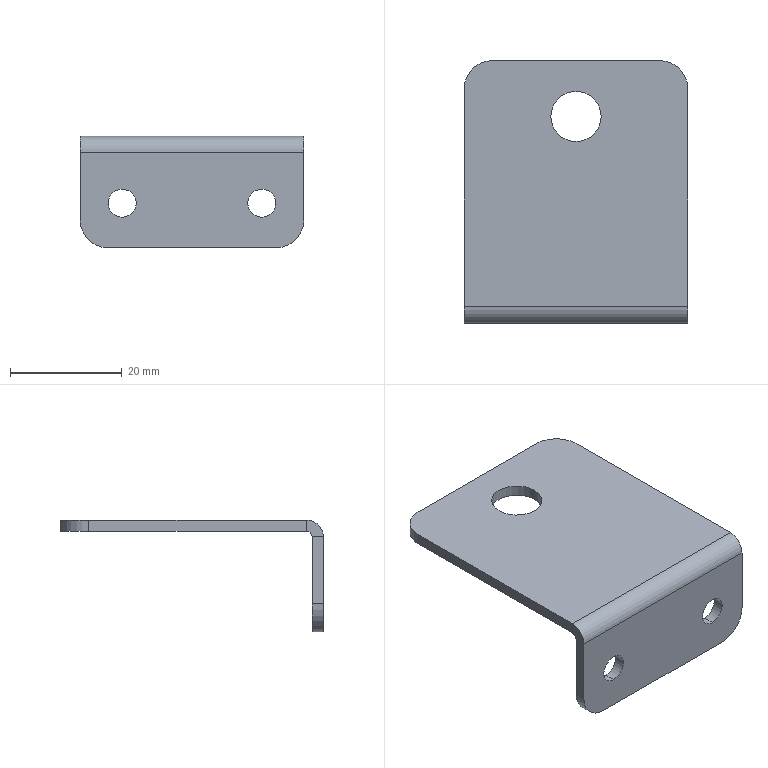Part | SolidWorks | features BaseBody 1 | 1 solid | 24 faces | box 40 x 47 x 20 mm | volume 4883 mm3 | cylinder 12 | plane 12 | commonest cylinder face diameters 5 x4 10 x4 9 x2 2 x1 6 x1
STEP:
#1=CARTESIAN_POINT('',(-12.5,-21.5,-9.5));
#2=VERTEX_POINT('',#1);
#3=CARTESIAN_POINT('',(-12.5,-23.5,-9.5));
#4=VERTEX_POINT('',#3);
#5=CARTESIAN_POINT('',(-12.5,-21.5,-9.5));
#6=DIRECTION('',(0.,-1.,0.));
#7=VECTOR('',#6,1000.);
#8=LINE('',#5,#7);
#9=EDGE_CURVE('',#2,#4,#8,.T.);
#10=ORIENTED_EDGE('',*,*,#9,.F.);
#11=CARTESIAN_POINT('',(-12.5,-21.5,-14.5));
#12=VERTEX_POINT('',#11);
#13=CARTESIAN_POINT('',(-12.5,-21.5,-12.));
#14=DIRECTION('',(0.,-1.,0.));
#15=DIRECTION('',(0.,0.,-1.));
#16=AXIS2_PLACEMENT_3D('',#13,#14,#15);
#17=CIRCLE('',#16,2.5);
#18=EDGE_CURVE('',#12,#2,#17,.T.);
#19=ORIENTED_EDGE('',*,*,#18,.F.);
#20=CARTESIAN_POINT('',(-12.5,-23.5,-14.5));
#21=VERTEX_POINT('',#20);
#22=CARTESIAN_POINT('',(-12.5,-21.5,-14.5));
#23=DIRECTION('',(0.,-1.,0.));
#24=VECTOR('',#23,1000.);
#25=LINE('',#22,#24);
#26=EDGE_CURVE('',#12,#21,#25,.T.);
#27=ORIENTED_EDGE('',*,*,#26,.T.);
#28=CARTESIAN_POINT('',(-12.5,-23.5,-12.));
#29=DIRECTION('',(0.,-1.,0.));
#30=DIRECTION('',(0.,0.,-1.));
#31=AXIS2_PLACEMENT_3D('',#28,#29,#30);
#32=CIRCLE('',#31,2.5);
#33=EDGE_CURVE('',#21,#4,#32,.T.);
#34=ORIENTED_EDGE('',*,*,#33,.T.);
#35=EDGE_LOOP('',(#10,#19,#27,#34));
#36=FACE_OUTER_BOUND('',#35,.T.);
#37=CARTESIAN_POINT('',(-12.5,-21.5,-12.));
#38=DIRECTION('',(0.,-1.,0.));
#39=DIRECTION('',(0.,0.,-1.));
#40=AXIS2_PLACEMENT_3D('',#37,#38,#39);
#41=CYLINDRICAL_SURFACE('',#40,2.5);
#42=ADVANCED_FACE('',(#36),#41,.F.);
#43=CARTESIAN_POINT('',(12.5,-21.5,-9.5));
#44=VERTEX_POINT('',#43);
#45=CARTESIAN_POINT('',(12.5,-23.5,-9.5));
#46=VERTEX_POINT('',#45);
#47=CARTESIAN_POINT('',(12.5,-21.5,-9.5));
#48=DIRECTION('',(0.,-1.,0.));
#49=VECTOR('',#48,1000.);
#50=LINE('',#47,#49);
#51=EDGE_CURVE('',#44,#46,#50,.T.);
#52=ORIENTED_EDGE('',*,*,#51,.F.);
#53=CARTESIAN_POINT('',(12.5,-21.5,-14.5));
#54=VERTEX_POINT('',#53);
#55=CARTESIAN_POINT('',(12.5,-21.5,-12.));
#56=DIRECTION('',(0.,-1.,0.));
#57=DIRECTION('',(0.,0.,1.));
#58=AXIS2_PLACEMENT_3D('',#55,#56,#57);
#59=CIRCLE('',#58,2.5);
#60=EDGE_CURVE('',#54,#44,#59,.T.);
#61=ORIENTED_EDGE('',*,*,#60,.F.);
#62=CARTESIAN_POINT('',(12.5,-23.5,-14.5));
#63=VERTEX_POINT('',#62);
#64=CARTESIAN_POINT('',(12.5,-21.5,-14.5));
#65=DIRECTION('',(0.,-1.,0.));
#66=VECTOR('',#65,1000.);
#67=LINE('',#64,#66);
#68=EDGE_CURVE('',#54,#63,#67,.T.);
#69=ORIENTED_EDGE('',*,*,#68,.T.);
#70=CARTESIAN_POINT('',(12.5,-23.5,-12.));
#71=DIRECTION('',(0.,-1.,0.));
#72=DIRECTION('',(0.,0.,1.));
#73=AXIS2_PLACEMENT_3D('',#70,#71,#72);
#74=CIRCLE('',#73,2.5);
#75=EDGE_CURVE('',#63,#46,#74,.T.);
#76=ORIENTED_EDGE('',*,*,#75,.T.);
#77=EDGE_LOOP('',(#52,#61,#69,#76));
#78=FACE_OUTER_BOUND('',#77,.T.);
#79=CARTESIAN_POINT('',(12.5,-21.5,-12.));
#80=DIRECTION('',(0.,-1.,0.));
#81=DIRECTION('',(0.,0.,-1.));
#82=AXIS2_PLACEMENT_3D('',#79,#80,#81);
#83=CYLINDRICAL_SURFACE('',#82,2.5);
#84=ADVANCED_FACE('',(#78),#83,.F.);
#85=CARTESIAN_POINT('',(-4.5,13.5,-2.));
#86=VERTEX_POINT('',#85);
#87=CARTESIAN_POINT('',(-4.5,13.5,0.));
#88=VERTEX_POINT('',#87);
#89=CARTESIAN_POINT('',(-4.5,13.5,-2.));
#90=DIRECTION('',(0.,0.,1.));
#91=VECTOR('',#90,1000.);
#92=LINE('',#89,#91);
#93=EDGE_CURVE('',#86,#88,#92,.T.);
#94=ORIENTED_EDGE('',*,*,#93,.F.);
#95=CARTESIAN_POINT('',(4.5,13.5,-2.));
#96=VERTEX_POINT('',#95);
#97=CARTESIAN_POINT('',(0.,13.5,-2.));
#98=DIRECTION('',(0.,0.,1.));
#99=DIRECTION('',(1.,0.,0.));
#100=AXIS2_PLACEMENT_3D('',#97,#98,#99);
#101=CIRCLE('',#100,4.5);
#102=EDGE_CURVE('',#96,#86,#101,.T.);
#103=ORIENTED_EDGE('',*,*,#102,.F.);
#104=CARTESIAN_POINT('',(4.5,13.5,0.));
#105=VERTEX_POINT('',#104);
#106=CARTESIAN_POINT('',(4.5,13.5,-2.));
#107=DIRECTION('',(0.,0.,1.));
#108=VECTOR('',#107,1000.);
#109=LINE('',#106,#108);
#110=EDGE_CURVE('',#96,#105,#109,.T.);
#111=ORIENTED_EDGE('',*,*,#110,.T.);
#112=CARTESIAN_POINT('',(0.,13.5,0.));
#113=DIRECTION('',(0.,0.,1.));
#114=DIRECTION('',(1.,0.,0.));
#115=AXIS2_PLACEMENT_3D('',#112,#113,#114);
#116=CIRCLE('',#115,4.5);
#117=EDGE_CURVE('',#105,#88,#116,.T.);
#118=ORIENTED_EDGE('',*,*,#117,.T.);
#119=EDGE_LOOP('',(#94,#103,#111,#118));
#120=FACE_OUTER_BOUND('',#119,.T.);
#121=CARTESIAN_POINT('',(0.,13.5,-2.));
#122=DIRECTION('',(0.,0.,1.));
#123=DIRECTION('',(1.,0.,0.));
#124=AXIS2_PLACEMENT_3D('',#121,#122,#123);
#125=CYLINDRICAL_SURFACE('',#124,4.5);
#126=ADVANCED_FACE('',(#120),#125,.F.);
#127=CARTESIAN_POINT('',(-20.,18.5,-2.));
#128=VERTEX_POINT('',#127);
#129=CARTESIAN_POINT('',(-15.,23.5,-2.));
#130=VERTEX_POINT('',#129);
#131=CARTESIAN_POINT('',(-15.,18.5,-2.));
#132=DIRECTION('',(0.,0.,-1.));
#133=DIRECTION('',(-1.,0.,0.));
#134=AXIS2_PLACEMENT_3D('',#131,#132,#133);
#135=CIRCLE('',#134,5.);
#136=EDGE_CURVE('',#128,#130,#135,.T.);
#137=ORIENTED_EDGE('',*,*,#136,.F.);
#138=CARTESIAN_POINT('',(-20.,18.5,0.));
#139=VERTEX_POINT('',#138);
#140=CARTESIAN_POINT('',(-20.,18.5,-2.));
#141=DIRECTION('',(0.,0.,-1.));
#142=VECTOR('',#141,1000.);
#143=LINE('',#140,#142);
#144=EDGE_CURVE('',#139,#128,#143,.T.);
#145=ORIENTED_EDGE('',*,*,#144,.F.);
#146=CARTESIAN_POINT('',(-15.,23.5,0.));
#147=VERTEX_POINT('',#146);
#148=CARTESIAN_POINT('',(-15.,18.5,0.));
#149=DIRECTION('',(0.,0.,1.));
#150=DIRECTION('',(-1.,0.,0.));
#151=AXIS2_PLACEMENT_3D('',#148,#149,#150);
#152=CIRCLE('',#151,5.);
#153=EDGE_CURVE('',#147,#139,#152,.T.);
#154=ORIENTED_EDGE('',*,*,#153,.F.);
#155=CARTESIAN_POINT('',(-15.,23.5,-2.));
#156=DIRECTION('',(0.,0.,1.));
#157=VECTOR('',#156,1000.);
#158=LINE('',#155,#157);
#159=EDGE_CURVE('',#130,#147,#158,.T.);
#160=ORIENTED_EDGE('',*,*,#159,.F.);
#161=EDGE_LOOP('',(#137,#145,#154,#160));
#162=FACE_OUTER_BOUND('',#161,.T.);
#163=CARTESIAN_POINT('',(-15.,18.5,-2.));
#164=DIRECTION('',(0.,0.,1.));
#165=DIRECTION('',(1.,0.,0.));
#166=AXIS2_PLACEMENT_3D('',#163,#164,#165);
#167=CYLINDRICAL_SURFACE('',#166,5.);
#168=ADVANCED_FACE('',(#162),#167,.T.);
#169=CARTESIAN_POINT('',(15.,23.5,-2.));
#170=VERTEX_POINT('',#169);
#171=CARTESIAN_POINT('',(20.,18.5,-2.));
#172=VERTEX_POINT('',#171);
#173=CARTESIAN_POINT('',(15.,18.5,-2.));
#174=DIRECTION('',(0.,0.,-1.));
#175=DIRECTION('',(-1.,0.,0.));
#176=AXIS2_PLACEMENT_3D('',#173,#174,#175);
#177=CIRCLE('',#176,5.);
#178=EDGE_CURVE('',#170,#172,#177,.T.);
#179=ORIENTED_EDGE('',*,*,#178,.F.);
#180=CARTESIAN_POINT('',(15.,23.5,0.));
#181=VERTEX_POINT('',#180);
#182=CARTESIAN_POINT('',(15.,23.5,-2.));
#183=DIRECTION('',(0.,0.,-1.));
#184=VECTOR('',#183,1000.);
#185=LINE('',#182,#184);
#186=EDGE_CURVE('',#181,#170,#185,.T.);
#187=ORIENTED_EDGE('',*,*,#186,.F.);
#188=CARTESIAN_POINT('',(20.,18.5,0.));
#189=VERTEX_POINT('',#188);
#190=CARTESIAN_POINT('',(15.,18.5,0.));
#191=DIRECTION('',(0.,0.,1.));
#192=DIRECTION('',(-1.,0.,0.));
#193=AXIS2_PLACEMENT_3D('',#190,#191,#192);
#194=CIRCLE('',#193,5.);
#195=EDGE_CURVE('',#189,#181,#194,.T.);
#196=ORIENTED_EDGE('',*,*,#195,.F.);
#197=CARTESIAN_POINT('',(20.,18.5,-2.));
#198=DIRECTION('',(0.,0.,1.));
#199=VECTOR('',#198,1000.);
#200=LINE('',#197,#199);
#201=EDGE_CURVE('',#172,#189,#200,.T.);
#202=ORIENTED_EDGE('',*,*,#201,.F.);
#203=EDGE_LOOP('',(#179,#187,#196,#202));
#204=FACE_OUTER_BOUND('',#203,.T.);
#205=CARTESIAN_POINT('',(15.,18.5,-2.));
#206=DIRECTION('',(0.,0.,1.));
#207=DIRECTION('',(1.,0.,0.));
#208=AXIS2_PLACEMENT_3D('',#205,#206,#207);
#209=CYLINDRICAL_SURFACE('',#208,5.);
#210=ADVANCED_FACE('',(#204),#209,.T.);
#211=CARTESIAN_POINT('',(-20.,-23.5,-15.));
#212=VERTEX_POINT('',#211);
#213=CARTESIAN_POINT('',(-15.,-23.5,-20.));
#214=VERTEX_POINT('',#213);
#215=CARTESIAN_POINT('',(-15.,-23.5,-15.));
#216=DIRECTION('',(0.,-1.,0.));
#217=DIRECTION('',(0.,0.,1.));
#218=AXIS2_PLACEMENT_3D('',#215,#216,#217);
#219=CIRCLE('',#218,5.);
#220=EDGE_CURVE('',#212,#214,#219,.T.);
#221=ORIENTED_EDGE('',*,*,#220,.F.);
#222=CARTESIAN_POINT('',(-20.,-21.5,-15.));
#223=VERTEX_POINT('',#222);
#224=CARTESIAN_POINT('',(-20.,-23.5,-15.));
#225=DIRECTION('',(0.,-1.,0.));
#226=VECTOR('',#225,1000.);
#227=LINE('',#224,#226);
#228=EDGE_CURVE('',#223,#212,#227,.T.);
#229=ORIENTED_EDGE('',*,*,#228,.F.);
#230=CARTESIAN_POINT('',(-15.,-21.5,-20.));
#231=VERTEX_POINT('',#230);
#232=CARTESIAN_POINT('',(-15.,-21.5,-15.));
#233=DIRECTION('',(0.,1.,0.));
#234=DIRECTION('',(0.,0.,1.));
#235=AXIS2_PLACEMENT_3D('',#232,#233,#234);
#236=CIRCLE('',#235,5.);
#237=EDGE_CURVE('',#231,#223,#236,.T.);
#238=ORIENTED_EDGE('',*,*,#237,.F.);
#239=CARTESIAN_POINT('',(-15.,-23.5,-20.));
#240=DIRECTION('',(0.,1.,0.));
#241=VECTOR('',#240,1000.);
#242=LINE('',#239,#241);
#243=EDGE_CURVE('',#214,#231,#242,.T.);
#244=ORIENTED_EDGE('',*,*,#243,.F.);
#245=EDGE_LOOP('',(#221,#229,#238,#244));
#246=FACE_OUTER_BOUND('',#245,.T.);
#247=CARTESIAN_POINT('',(-15.,-23.5,-15.));
#248=DIRECTION('',(0.,1.,0.));
#249=DIRECTION('',(0.,0.,1.));
#250=AXIS2_PLACEMENT_3D('',#247,#248,#249);
#251=CYLINDRICAL_SURFACE('',#250,5.);
#252=ADVANCED_FACE('',(#246),#251,.T.);
#253=CARTESIAN_POINT('',(15.,-23.5,-20.));
#254=VERTEX_POINT('',#253);
#255=CARTESIAN_POINT('',(20.,-23.5,-15.));
#256=VERTEX_POINT('',#255);
#257=CARTESIAN_POINT('',(15.,-23.5,-15.));
#258=DIRECTION('',(0.,-1.,0.));
#259=DIRECTION('',(0.,0.,1.));
#260=AXIS2_PLACEMENT_3D('',#257,#258,#259);
#261=CIRCLE('',#260,5.);
#262=EDGE_CURVE('',#254,#256,#261,.T.);
#263=ORIENTED_EDGE('',*,*,#262,.F.);
#264=CARTESIAN_POINT('',(15.,-21.5,-20.));
#265=VERTEX_POINT('',#264);
#266=CARTESIAN_POINT('',(15.,-23.5,-20.));
#267=DIRECTION('',(0.,-1.,0.));
#268=VECTOR('',#267,1000.);
#269=LINE('',#266,#268);
#270=EDGE_CURVE('',#265,#254,#269,.T.);
#271=ORIENTED_EDGE('',*,*,#270,.F.);
#272=CARTESIAN_POINT('',(20.,-21.5,-15.));
#273=VERTEX_POINT('',#272);
#274=CARTESIAN_POINT('',(15.,-21.5,-15.));
#275=DIRECTION('',(0.,1.,0.));
#276=DIRECTION('',(0.,0.,1.));
#277=AXIS2_PLACEMENT_3D('',#274,#275,#276);
#278=CIRCLE('',#277,5.);
#279=EDGE_CURVE('',#273,#265,#278,.T.);
#280=ORIENTED_EDGE('',*,*,#279,.F.);
#281=CARTESIAN_POINT('',(20.,-23.5,-15.));
#282=DIRECTION('',(0.,1.,0.));
#283=VECTOR('',#282,1000.);
#284=LINE('',#281,#283);
#285=EDGE_CURVE('',#256,#273,#284,.T.);
#286=ORIENTED_EDGE('',*,*,#285,.F.);
#287=EDGE_LOOP('',(#263,#271,#280,#286));
#288=FACE_OUTER_BOUND('',#287,.T.);
#289=CARTESIAN_POINT('',(15.,-23.5,-15.));
#290=DIRECTION('',(0.,1.,0.));
#291=DIRECTION('',(0.,0.,1.));
#292=AXIS2_PLACEMENT_3D('',#289,#290,#291);
#293=CYLINDRICAL_SURFACE('',#292,5.);
#294=ADVANCED_FACE('',(#288),#293,.T.);
#295=CARTESIAN_POINT('',(20.,-21.5,-20.));
#296=DIRECTION('',(1.,0.,0.));
#297=VECTOR('',#296,1000.);
#298=LINE('',#295,#297);
#299=EDGE_CURVE('',#231,#265,#298,.T.);
#300=ORIENTED_EDGE('',*,*,#299,.T.);
#301=ORIENTED_EDGE('',*,*,#270,.T.);
#302=CARTESIAN_POINT('',(0.,-23.5,-20.));
#303=DIRECTION('',(1.,0.,0.));
#304=VECTOR('',#303,1000.);
#305=LINE('',#302,#304);
#306=EDGE_CURVE('',#214,#254,#305,.T.);
#307=ORIENTED_EDGE('',*,*,#306,.F.);
#308=ORIENTED_EDGE('',*,*,#243,.T.);
#309=EDGE_LOOP('',(#300,#301,#307,#308));
#310=FACE_OUTER_BOUND('',#309,.T.);
#311=CARTESIAN_POINT('',(20.,-23.5,-20.));
#312=DIRECTION('',(0.,0.,1.));
#313=DIRECTION('',(0.,-1.,0.));
#314=AXIS2_PLACEMENT_3D('',#311,#312,#313);
#315=PLANE('',#314);
#316=ADVANCED_FACE('',(#310),#315,.F.);
#317=ORIENTED_EDGE('',*,*,#60,.T.);
#318=CARTESIAN_POINT('',(12.5,-21.5,-12.));
#319=DIRECTION('',(0.,-1.,0.));
#320=DIRECTION('',(0.,0.,1.));
#321=AXIS2_PLACEMENT_3D('',#318,#319,#320);
#322=CIRCLE('',#321,2.5);
#323=EDGE_CURVE('',#44,#54,#322,.T.);
#324=ORIENTED_EDGE('',*,*,#323,.T.);
#325=EDGE_LOOP('',(#317,#324));
#326=FACE_BOUND('',#325,.T.);
#327=ORIENTED_EDGE('',*,*,#18,.T.);
#328=CARTESIAN_POINT('',(-12.5,-21.5,-12.));
#329=DIRECTION('',(0.,-1.,0.));
#330=DIRECTION('',(0.,0.,-1.));
#331=AXIS2_PLACEMENT_3D('',#328,#329,#330);
#332=CIRCLE('',#331,2.5);
#333=EDGE_CURVE('',#2,#12,#332,.T.);
#334=ORIENTED_EDGE('',*,*,#333,.T.);
#335=EDGE_LOOP('',(#327,#334));
#336=FACE_BOUND('',#335,.T.);
#337=CARTESIAN_POINT('',(20.,-21.5,-3.));
#338=VERTEX_POINT('',#337);
#339=CARTESIAN_POINT('',(20.,-21.5,-2.));
#340=DIRECTION('',(0.,0.,1.));
#341=VECTOR('',#340,1000.);
#342=LINE('',#339,#341);
#343=EDGE_CURVE('',#273,#338,#342,.T.);
#344=ORIENTED_EDGE('',*,*,#343,.F.);
#345=ORIENTED_EDGE('',*,*,#279,.T.);
#346=ORIENTED_EDGE('',*,*,#299,.F.);
#347=ORIENTED_EDGE('',*,*,#237,.T.);
#348=CARTESIAN_POINT('',(-20.,-21.5,-3.));
#349=VERTEX_POINT('',#348);
#350=CARTESIAN_POINT('',(-20.,-21.5,-20.));
#351=DIRECTION('',(0.,0.,-1.));
#352=VECTOR('',#351,1000.);
#353=LINE('',#350,#352);
#354=EDGE_CURVE('',#349,#223,#353,.T.);
#355=ORIENTED_EDGE('',*,*,#354,.F.);
#356=CARTESIAN_POINT('',(20.,-21.5,-3.));
#357=DIRECTION('',(-1.,0.,0.));
#358=VECTOR('',#357,1000.);
#359=LINE('',#356,#358);
#360=EDGE_CURVE('',#338,#349,#359,.T.);
#361=ORIENTED_EDGE('',*,*,#360,.F.);
#362=EDGE_LOOP('',(#344,#345,#346,#347,#355,#361));
#363=FACE_OUTER_BOUND('',#362,.T.);
#364=CARTESIAN_POINT('',(0.,-21.5,0.));
#365=DIRECTION('',(0.,1.,0.));
#366=DIRECTION('',(0.,0.,-1.));
#367=AXIS2_PLACEMENT_3D('',#364,#365,#366);
#368=PLANE('',#367);
#369=ADVANCED_FACE('',(#326,#336,#363),#368,.T.);
#370=ORIENTED_EDGE('',*,*,#75,.F.);
#371=CARTESIAN_POINT('',(12.5,-23.5,-12.));
#372=DIRECTION('',(0.,-1.,0.));
#373=DIRECTION('',(0.,0.,1.));
#374=AXIS2_PLACEMENT_3D('',#371,#372,#373);
#375=CIRCLE('',#374,2.5);
#376=EDGE_CURVE('',#46,#63,#375,.T.);
#377=ORIENTED_EDGE('',*,*,#376,.F.);
#378=EDGE_LOOP('',(#370,#377));
#379=FACE_BOUND('',#378,.T.);
#380=ORIENTED_EDGE('',*,*,#33,.F.);
#381=CARTESIAN_POINT('',(-12.5,-23.5,-12.));
#382=DIRECTION('',(0.,-1.,0.));
#383=DIRECTION('',(0.,0.,-1.));
#384=AXIS2_PLACEMENT_3D('',#381,#382,#383);
#385=CIRCLE('',#384,2.5);
#386=EDGE_CURVE('',#4,#21,#385,.T.);
#387=ORIENTED_EDGE('',*,*,#386,.F.);
#388=EDGE_LOOP('',(#380,#387));
#389=FACE_BOUND('',#388,.T.);
#390=ORIENTED_EDGE('',*,*,#306,.T.);
#391=ORIENTED_EDGE('',*,*,#262,.T.);
#392=CARTESIAN_POINT('',(20.,-23.5,-3.));
#393=VERTEX_POINT('',#392);
#394=CARTESIAN_POINT('',(20.,-23.5,0.));
#395=DIRECTION('',(0.,0.,1.));
#396=VECTOR('',#395,1000.);
#397=LINE('',#394,#396);
#398=EDGE_CURVE('',#256,#393,#397,.T.);
#399=ORIENTED_EDGE('',*,*,#398,.T.);
#400=CARTESIAN_POINT('',(-20.,-23.5,-3.));
#401=VERTEX_POINT('',#400);
#402=CARTESIAN_POINT('',(20.,-23.5,-3.));
#403=DIRECTION('',(1.,0.,0.));
#404=VECTOR('',#403,1000.);
#405=LINE('',#402,#404);
#406=EDGE_CURVE('',#401,#393,#405,.T.);
#407=ORIENTED_EDGE('',*,*,#406,.F.);
#408=CARTESIAN_POINT('',(-20.,-23.5,0.));
#409=DIRECTION('',(0.,0.,-1.));
#410=VECTOR('',#409,1000.);
#411=LINE('',#408,#410);
#412=EDGE_CURVE('',#401,#212,#411,.T.);
#413=ORIENTED_EDGE('',*,*,#412,.T.);
#414=ORIENTED_EDGE('',*,*,#220,.T.);
#415=EDGE_LOOP('',(#390,#391,#399,#407,#413,#414));
#416=FACE_OUTER_BOUND('',#415,.T.);
#417=CARTESIAN_POINT('',(0.,-23.5,0.));
#418=DIRECTION('',(0.,1.,0.));
#419=DIRECTION('',(0.,0.,-1.));
#420=AXIS2_PLACEMENT_3D('',#417,#418,#419);
#421=PLANE('',#420);
#422=ADVANCED_FACE('',(#379,#389,#416),#421,.F.);
#423=ORIENTED_EDGE('',*,*,#398,.F.);
#424=ORIENTED_EDGE('',*,*,#285,.T.);
#425=ORIENTED_EDGE('',*,*,#343,.T.);
#426=CARTESIAN_POINT('',(20.,-23.5,-3.));
#427=DIRECTION('',(0.,-1.,0.));
#428=VECTOR('',#427,1000.);
#429=LINE('',#426,#428);
#430=EDGE_CURVE('',#338,#393,#429,.T.);
#431=ORIENTED_EDGE('',*,*,#430,.T.);
#432=EDGE_LOOP('',(#423,#424,#425,#431));
#433=FACE_OUTER_BOUND('',#432,.T.);
#434=CARTESIAN_POINT('',(20.,-23.5,-2.));
#435=DIRECTION('',(-1.,0.,0.));
#436=DIRECTION('',(0.,0.,1.));
#437=AXIS2_PLACEMENT_3D('',#434,#435,#436);
#438=PLANE('',#437);
#439=ADVANCED_FACE('',(#433),#438,.F.);
#440=ORIENTED_EDGE('',*,*,#354,.T.);
#441=ORIENTED_EDGE('',*,*,#228,.T.);
#442=ORIENTED_EDGE('',*,*,#412,.F.);
#443=CARTESIAN_POINT('',(-20.,-21.5,-3.));
#444=DIRECTION('',(0.,-1.,0.));
#445=VECTOR('',#444,1000.);
#446=LINE('',#443,#445);
#447=EDGE_CURVE('',#349,#401,#446,.T.);
#448=ORIENTED_EDGE('',*,*,#447,.F.);
#449=EDGE_LOOP('',(#440,#441,#442,#448));
#450=FACE_OUTER_BOUND('',#449,.T.);
#451=CARTESIAN_POINT('',(-20.,-23.5,-20.));
#452=DIRECTION('',(1.,0.,0.));
#453=DIRECTION('',(0.,1.,0.));
#454=AXIS2_PLACEMENT_3D('',#451,#452,#453);
#455=PLANE('',#454);
#456=ADVANCED_FACE('',(#450),#455,.F.);
#457=CARTESIAN_POINT('',(-20.,-20.5,-2.));
#458=VERTEX_POINT('',#457);
#459=CARTESIAN_POINT('',(20.,-20.5,-2.));
#460=VERTEX_POINT('',#459);
#461=CARTESIAN_POINT('',(-20.,-20.5,-2.));
#462=DIRECTION('',(1.,0.,0.));
#463=VECTOR('',#462,1000.);
#464=LINE('',#461,#463);
#465=EDGE_CURVE('',#458,#460,#464,.T.);
#466=ORIENTED_EDGE('',*,*,#465,.T.);
#467=CARTESIAN_POINT('',(20.,-20.5,-3.));
#468=DIRECTION('',(1.,0.,0.));
#469=DIRECTION('',(0.,0.,1.));
#470=AXIS2_PLACEMENT_3D('',#467,#468,#469);
#471=CIRCLE('',#470,1.);
#472=EDGE_CURVE('',#460,#338,#471,.T.);
#473=ORIENTED_EDGE('',*,*,#472,.T.);
#474=ORIENTED_EDGE('',*,*,#360,.T.);
#475=CARTESIAN_POINT('',(-20.,-20.5,-3.));
#476=DIRECTION('',(-1.,0.,0.));
#477=DIRECTION('',(0.,0.,1.));
#478=AXIS2_PLACEMENT_3D('',#475,#476,#477);
#479=CIRCLE('',#478,1.);
#480=EDGE_CURVE('',#349,#458,#479,.T.);
#481=ORIENTED_EDGE('',*,*,#480,.T.);
#482=EDGE_LOOP('',(#466,#473,#474,#481));
#483=FACE_OUTER_BOUND('',#482,.T.);
#484=CARTESIAN_POINT('',(-20.,-20.5,-3.));
#485=DIRECTION('',(-1.,0.,0.));
#486=DIRECTION('',(0.,-1.,0.));
#487=AXIS2_PLACEMENT_3D('',#484,#485,#486);
#488=CYLINDRICAL_SURFACE('',#487,1.);
#489=ADVANCED_FACE('',(#483),#488,.F.);
#490=CARTESIAN_POINT('',(-20.,-20.5,0.));
#491=VERTEX_POINT('',#490);
#492=CARTESIAN_POINT('',(20.,-20.5,0.));
#493=VERTEX_POINT('',#492);
#494=CARTESIAN_POINT('',(-20.,-20.5,0.));
#495=DIRECTION('',(1.,0.,0.));
#496=VECTOR('',#495,1000.);
#497=LINE('',#494,#496);
#498=EDGE_CURVE('',#491,#493,#497,.T.);
#499=ORIENTED_EDGE('',*,*,#498,.F.);
#500=CARTESIAN_POINT('',(-20.,-20.5,-3.));
#501=DIRECTION('',(-1.,0.,0.));
#502=DIRECTION('',(0.,0.,1.));
#503=AXIS2_PLACEMENT_3D('',#500,#501,#502);
#504=CIRCLE('',#503,3.);
#505=EDGE_CURVE('',#401,#491,#504,.T.);
#506=ORIENTED_EDGE('',*,*,#505,.F.);
#507=ORIENTED_EDGE('',*,*,#406,.T.);
#508=CARTESIAN_POINT('',(20.,-20.5,-3.));
#509=DIRECTION('',(1.,0.,0.));
#510=DIRECTION('',(0.,0.,1.));
#511=AXIS2_PLACEMENT_3D('',#508,#509,#510);
#512=CIRCLE('',#511,3.);
#513=EDGE_CURVE('',#493,#393,#512,.T.);
#514=ORIENTED_EDGE('',*,*,#513,.F.);
#515=EDGE_LOOP('',(#499,#506,#507,#514));
#516=FACE_OUTER_BOUND('',#515,.T.);
#517=CARTESIAN_POINT('',(-20.,-20.5,-3.));
#518=DIRECTION('',(-1.,0.,0.));
#519=DIRECTION('',(0.,-1.,0.));
#520=AXIS2_PLACEMENT_3D('',#517,#518,#519);
#521=CYLINDRICAL_SURFACE('',#520,3.);
#522=ADVANCED_FACE('',(#516),#521,.T.);
#523=ORIENTED_EDGE('',*,*,#480,.F.);
#524=ORIENTED_EDGE('',*,*,#447,.T.);
#525=ORIENTED_EDGE('',*,*,#505,.T.);
#526=CARTESIAN_POINT('',(-20.,-20.5,-2.));
#527=DIRECTION('',(0.,0.,1.));
#528=VECTOR('',#527,1000.);
#529=LINE('',#526,#528);
#530=EDGE_CURVE('',#458,#491,#529,.T.);
#531=ORIENTED_EDGE('',*,*,#530,.F.);
#532=EDGE_LOOP('',(#523,#524,#525,#531));
#533=FACE_OUTER_BOUND('',#532,.T.);
#534=CARTESIAN_POINT('',(-20.,-20.5,-3.));
#535=DIRECTION('',(1.,0.,0.));
#536=DIRECTION('',(0.,1.,0.));
#537=AXIS2_PLACEMENT_3D('',#534,#535,#536);
#538=PLANE('',#537);
#539=ADVANCED_FACE('',(#533),#538,.F.);
#540=ORIENTED_EDGE('',*,*,#430,.F.);
#541=ORIENTED_EDGE('',*,*,#472,.F.);
#542=CARTESIAN_POINT('',(20.,-20.5,-2.));
#543=DIRECTION('',(0.,0.,1.));
#544=VECTOR('',#543,1000.);
#545=LINE('',#542,#544);
#546=EDGE_CURVE('',#460,#493,#545,.T.);
#547=ORIENTED_EDGE('',*,*,#546,.T.);
#548=ORIENTED_EDGE('',*,*,#513,.T.);
#549=EDGE_LOOP('',(#540,#541,#547,#548));
#550=FACE_OUTER_BOUND('',#549,.T.);
#551=CARTESIAN_POINT('',(20.,-20.5,-3.));
#552=DIRECTION('',(1.,0.,0.));
#553=DIRECTION('',(0.,1.,0.));
#554=AXIS2_PLACEMENT_3D('',#551,#552,#553);
#555=PLANE('',#554);
#556=ADVANCED_FACE('',(#550),#555,.T.);
#557=CARTESIAN_POINT('',(20.,23.5,-2.));
#558=DIRECTION('',(0.,1.,0.));
#559=VECTOR('',#558,1000.);
#560=LINE('',#557,#559);
#561=EDGE_CURVE('',#460,#172,#560,.T.);
#562=ORIENTED_EDGE('',*,*,#561,.T.);
#563=ORIENTED_EDGE('',*,*,#201,.T.);
#564=CARTESIAN_POINT('',(20.,23.5,0.));
#565=DIRECTION('',(0.,1.,0.));
#566=VECTOR('',#565,1000.);
#567=LINE('',#564,#566);
#568=EDGE_CURVE('',#493,#189,#567,.T.);
#569=ORIENTED_EDGE('',*,*,#568,.F.);
#570=ORIENTED_EDGE('',*,*,#546,.F.);
#571=EDGE_LOOP('',(#562,#563,#569,#570));
#572=FACE_OUTER_BOUND('',#571,.T.);
#573=CARTESIAN_POINT('',(20.,23.5,-2.));
#574=DIRECTION('',(1.,0.,0.));
#575=DIRECTION('',(0.,1.,0.));
#576=AXIS2_PLACEMENT_3D('',#573,#574,#575);
#577=PLANE('',#576);
#578=ADVANCED_FACE('',(#572),#577,.T.);
#579=CARTESIAN_POINT('',(20.,23.5,0.));
#580=DIRECTION('',(-1.,0.,0.));
#581=VECTOR('',#580,1000.);
#582=LINE('',#579,#581);
#583=EDGE_CURVE('',#181,#147,#582,.T.);
#584=ORIENTED_EDGE('',*,*,#583,.F.);
#585=ORIENTED_EDGE('',*,*,#186,.T.);
#586=CARTESIAN_POINT('',(20.,23.5,-2.));
#587=DIRECTION('',(-1.,0.,0.));
#588=VECTOR('',#587,1000.);
#589=LINE('',#586,#588);
#590=EDGE_CURVE('',#170,#130,#589,.T.);
#591=ORIENTED_EDGE('',*,*,#590,.T.);
#592=ORIENTED_EDGE('',*,*,#159,.T.);
#593=EDGE_LOOP('',(#584,#585,#591,#592));
#594=FACE_OUTER_BOUND('',#593,.T.);
#595=CARTESIAN_POINT('',(20.,23.5,-2.));
#596=DIRECTION('',(0.,1.,0.));
#597=DIRECTION('',(1.,0.,0.));
#598=AXIS2_PLACEMENT_3D('',#595,#596,#597);
#599=PLANE('',#598);
#600=ADVANCED_FACE('',(#594),#599,.T.);
#601=ORIENTED_EDGE('',*,*,#117,.F.);
#602=CARTESIAN_POINT('',(0.,13.5,0.));
#603=DIRECTION('',(0.,0.,1.));
#604=DIRECTION('',(1.,0.,0.));
#605=AXIS2_PLACEMENT_3D('',#602,#603,#604);
#606=CIRCLE('',#605,4.5);
#607=EDGE_CURVE('',#88,#105,#606,.T.);
#608=ORIENTED_EDGE('',*,*,#607,.F.);
#609=EDGE_LOOP('',(#601,#608));
#610=FACE_BOUND('',#609,.T.);
#611=ORIENTED_EDGE('',*,*,#568,.T.);
#612=ORIENTED_EDGE('',*,*,#195,.T.);
#613=ORIENTED_EDGE('',*,*,#583,.T.);
#614=ORIENTED_EDGE('',*,*,#153,.T.);
#615=CARTESIAN_POINT('',(-20.,23.5,0.));
#616=DIRECTION('',(0.,-1.,0.));
#617=VECTOR('',#616,1000.);
#618=LINE('',#615,#617);
#619=EDGE_CURVE('',#139,#491,#618,.T.);
#620=ORIENTED_EDGE('',*,*,#619,.T.);
#621=ORIENTED_EDGE('',*,*,#498,.T.);
#622=EDGE_LOOP('',(#611,#612,#613,#614,#620,#621));
#623=FACE_OUTER_BOUND('',#622,.T.);
#624=CARTESIAN_POINT('',(0.,0.,0.));
#625=DIRECTION('',(0.,0.,-1.));
#626=DIRECTION('',(0.,-1.,0.));
#627=AXIS2_PLACEMENT_3D('',#624,#625,#626);
#628=PLANE('',#627);
#629=ADVANCED_FACE('',(#610,#623),#628,.F.);
#630=ORIENTED_EDGE('',*,*,#102,.T.);
#631=CARTESIAN_POINT('',(0.,13.5,-2.));
#632=DIRECTION('',(0.,0.,1.));
#633=DIRECTION('',(1.,0.,0.));
#634=AXIS2_PLACEMENT_3D('',#631,#632,#633);
#635=CIRCLE('',#634,4.5);
#636=EDGE_CURVE('',#86,#96,#635,.T.);
#637=ORIENTED_EDGE('',*,*,#636,.T.);
#638=EDGE_LOOP('',(#630,#637));
#639=FACE_BOUND('',#638,.T.);
#640=ORIENTED_EDGE('',*,*,#590,.F.);
#641=ORIENTED_EDGE('',*,*,#178,.T.);
#642=ORIENTED_EDGE('',*,*,#561,.F.);
#643=ORIENTED_EDGE('',*,*,#465,.F.);
#644=CARTESIAN_POINT('',(-20.,23.5,-2.));
#645=DIRECTION('',(0.,-1.,0.));
#646=VECTOR('',#645,1000.);
#647=LINE('',#644,#646);
#648=EDGE_CURVE('',#128,#458,#647,.T.);
#649=ORIENTED_EDGE('',*,*,#648,.F.);
#650=ORIENTED_EDGE('',*,*,#136,.T.);
#651=EDGE_LOOP('',(#640,#641,#642,#643,#649,#650));
#652=FACE_OUTER_BOUND('',#651,.T.);
#653=CARTESIAN_POINT('',(0.,0.,-2.));
#654=DIRECTION('',(0.,0.,-1.));
#655=DIRECTION('',(0.,-1.,0.));
#656=AXIS2_PLACEMENT_3D('',#653,#654,#655);
#657=PLANE('',#656);
#658=ADVANCED_FACE('',(#639,#652),#657,.T.);
#659=ORIENTED_EDGE('',*,*,#619,.F.);
#660=ORIENTED_EDGE('',*,*,#144,.T.);
#661=ORIENTED_EDGE('',*,*,#648,.T.);
#662=ORIENTED_EDGE('',*,*,#530,.T.);
#663=EDGE_LOOP('',(#659,#660,#661,#662));
#664=FACE_OUTER_BOUND('',#663,.T.);
#665=CARTESIAN_POINT('',(-20.,23.5,-2.));
#666=DIRECTION('',(-1.,0.,0.));
#667=DIRECTION('',(0.,1.,0.));
#668=AXIS2_PLACEMENT_3D('',#665,#666,#667);
#669=PLANE('',#668);
#670=ADVANCED_FACE('',(#664),#669,.T.);
#671=ORIENTED_EDGE('',*,*,#636,.F.);
#672=ORIENTED_EDGE('',*,*,#93,.T.);
#673=ORIENTED_EDGE('',*,*,#607,.T.);
#674=ORIENTED_EDGE('',*,*,#110,.F.);
#675=EDGE_LOOP('',(#671,#672,#673,#674));
#676=FACE_OUTER_BOUND('',#675,.T.);
#677=CARTESIAN_POINT('',(0.,13.5,-2.));
#678=DIRECTION('',(0.,0.,1.));
#679=DIRECTION('',(1.,0.,0.));
#680=AXIS2_PLACEMENT_3D('',#677,#678,#679);
#681=CYLINDRICAL_SURFACE('',#680,4.5);
#682=ADVANCED_FACE('',(#676),#681,.F.);
#683=ORIENTED_EDGE('',*,*,#323,.F.);
#684=ORIENTED_EDGE('',*,*,#51,.T.);
#685=ORIENTED_EDGE('',*,*,#376,.T.);
#686=ORIENTED_EDGE('',*,*,#68,.F.);
#687=EDGE_LOOP('',(#683,#684,#685,#686));
#688=FACE_OUTER_BOUND('',#687,.T.);
#689=CARTESIAN_POINT('',(12.5,-21.5,-12.));
#690=DIRECTION('',(0.,-1.,0.));
#691=DIRECTION('',(0.,0.,-1.));
#692=AXIS2_PLACEMENT_3D('',#689,#690,#691);
#693=CYLINDRICAL_SURFACE('',#692,2.5);
#694=ADVANCED_FACE('',(#688),#693,.F.);
#695=ORIENTED_EDGE('',*,*,#333,.F.);
#696=ORIENTED_EDGE('',*,*,#9,.T.);
#697=ORIENTED_EDGE('',*,*,#386,.T.);
#698=ORIENTED_EDGE('',*,*,#26,.F.);
#699=EDGE_LOOP('',(#695,#696,#697,#698));
#700=FACE_OUTER_BOUND('',#699,.T.);
#701=CARTESIAN_POINT('',(-12.5,-21.5,-12.));
#702=DIRECTION('',(0.,-1.,0.));
#703=DIRECTION('',(0.,0.,-1.));
#704=AXIS2_PLACEMENT_3D('',#701,#702,#703);
#705=CYLINDRICAL_SURFACE('',#704,2.5);
#706=ADVANCED_FACE('',(#700),#705,.F.);
#707=CLOSED_SHELL('',(#42,#84,#126,#168,#210,#252,#294,#316,#369,#422,#439,#456,#489,#522,#539,#556,#578,#600,#629,#658,#670,#682,#694,#706));
#708=MANIFOLD_SOLID_BREP('',#707);
#709=CARTESIAN_POINT('',(0.,0.,0.));
#710=DIRECTION('',(0.,0.,1.));
#711=DIRECTION('',(1.,0.,0.));
#712=AXIS2_PLACEMENT_3D('',#709,#710,#711);
#713=(LENGTH_UNIT()NAMED_UNIT(*)SI_UNIT(.MILLI.,.METRE.));
#714=UNCERTAINTY_MEASURE_WITH_UNIT(LENGTH_MEASURE(0.00001),#713,'','');
#715=(NAMED_UNIT(*)PLANE_ANGLE_UNIT()SI_UNIT($,.RADIAN.));
#716=(NAMED_UNIT(*)SI_UNIT($,.STERADIAN.)SOLID_ANGLE_UNIT());
#717=(GEOMETRIC_REPRESENTATION_CONTEXT(3)GLOBAL_UNCERTAINTY_ASSIGNED_CONTEXT((#714))GLOBAL_UNIT_ASSIGNED_CONTEXT((#713,#715,#716))REPRESENTATION_CONTEXT('',''));
#718=ADVANCED_BREP_SHAPE_REPRESENTATION('',(#708,#712),#717);